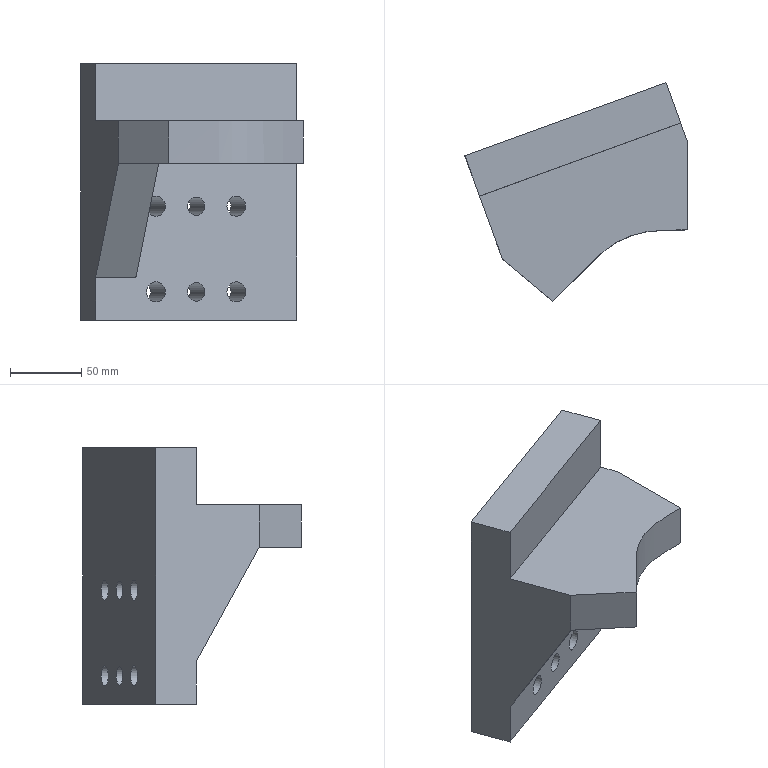Part | NX | features solid 2 | 1 solid | 20 faces | box 155.712 x 153.116 x 180 mm | volume 1134796 mm3 | plane 13 | cylinder 6 | spline 1 | commonest cylinder face diameters 14 x4 13 x2
STEP:
#1=CARTESIAN_POINT('',(-306.343,587.042,-175.));
#2=VERTEX_POINT('',#1);
#3=CARTESIAN_POINT('',(-300.235,589.265,-175.));
#4=DIRECTION('',(-0.342,0.9397,0.));
#5=DIRECTION('',(-0.9397,-0.342,0.));
#6=AXIS2_PLACEMENT_3D('',#3,#4,#5);
#7=CIRCLE('',#6,6.5);
#8=EDGE_CURVE('',#2,#2,#7,.F.);
#9=ORIENTED_EDGE('',*,*,#8,.T.);
#10=EDGE_LOOP('',(#9));
#11=FACE_BOUND('',#10,.T.);
#12=CARTESIAN_POINT('',(-278.622,597.132,-115.));
#13=VERTEX_POINT('',#12);
#14=CARTESIAN_POINT('',(-272.044,599.526,-115.));
#15=DIRECTION('',(-0.342,0.9397,0.));
#16=DIRECTION('',(-0.9397,-0.342,0.));
#17=AXIS2_PLACEMENT_3D('',#14,#15,#16);
#18=CIRCLE('',#17,7.);
#19=EDGE_CURVE('',#13,#13,#18,.F.);
#20=ORIENTED_EDGE('',*,*,#19,.T.);
#21=EDGE_LOOP('',(#20));
#22=FACE_BOUND('',#21,.T.);
#23=CARTESIAN_POINT('',(-335.003,576.611,-115.));
#24=VERTEX_POINT('',#23);
#25=CARTESIAN_POINT('',(-328.425,579.005,-115.));
#26=DIRECTION('',(-0.342,0.9397,0.));
#27=DIRECTION('',(-0.9397,-0.342,0.));
#28=AXIS2_PLACEMENT_3D('',#25,#26,#27);
#29=CIRCLE('',#28,7.);
#30=EDGE_CURVE('',#24,#24,#29,.F.);
#31=ORIENTED_EDGE('',*,*,#30,.T.);
#32=EDGE_LOOP('',(#31));
#33=FACE_BOUND('',#32,.T.);
#34=CARTESIAN_POINT('',(-370.712,563.614,-195.));
#35=VERTEX_POINT('',#34);
#36=CARTESIAN_POINT('',(-229.758,614.917,-195.));
#37=VERTEX_POINT('',#36);
#38=CARTESIAN_POINT('',(-389.448,556.794,-195.));
#39=DIRECTION('',(-0.9397,-0.342,0.));
#40=VECTOR('',#39,1000.);
#41=LINE('',#38,#40);
#42=EDGE_CURVE('',#35,#37,#41,.F.);
#43=ORIENTED_EDGE('',*,*,#42,.F.);
#44=CARTESIAN_POINT('',(-370.712,563.614,-15.));
#45=VERTEX_POINT('',#44);
#46=CARTESIAN_POINT('',(-370.712,563.614,-25.));
#47=DIRECTION('',(0.,0.,1.));
#48=VECTOR('',#47,1000.);
#49=LINE('',#46,#48);
#50=EDGE_CURVE('',#45,#35,#49,.F.);
#51=ORIENTED_EDGE('',*,*,#50,.F.);
#52=CARTESIAN_POINT('',(-229.758,614.917,-15.));
#53=VERTEX_POINT('',#52);
#54=CARTESIAN_POINT('',(-389.448,556.794,-15.));
#55=DIRECTION('',(0.9397,0.342,0.));
#56=VECTOR('',#55,1000.);
#57=LINE('',#54,#56);
#58=EDGE_CURVE('',#45,#53,#57,.T.);
#59=ORIENTED_EDGE('',*,*,#58,.T.);
#60=CARTESIAN_POINT('',(-229.758,614.917,-25.));
#61=DIRECTION('',(0.,0.,-1.));
#62=VECTOR('',#61,1000.);
#63=LINE('',#60,#62);
#64=EDGE_CURVE('',#53,#37,#63,.T.);
#65=ORIENTED_EDGE('',*,*,#64,.T.);
#66=EDGE_LOOP('',(#43,#51,#59,#65));
#67=FACE_BOUND('',#66,.T.);
#68=CARTESIAN_POINT('',(-306.343,587.042,-115.));
#69=VERTEX_POINT('',#68);
#70=CARTESIAN_POINT('',(-300.235,589.265,-115.));
#71=DIRECTION('',(-0.342,0.9397,0.));
#72=DIRECTION('',(-0.9397,-0.342,0.));
#73=AXIS2_PLACEMENT_3D('',#70,#71,#72);
#74=CIRCLE('',#73,6.5);
#75=EDGE_CURVE('',#69,#69,#74,.F.);
#76=ORIENTED_EDGE('',*,*,#75,.T.);
#77=EDGE_LOOP('',(#76));
#78=FACE_BOUND('',#77,.T.);
#79=CARTESIAN_POINT('',(-335.003,576.611,-175.));
#80=VERTEX_POINT('',#79);
#81=CARTESIAN_POINT('',(-328.425,579.005,-175.));
#82=DIRECTION('',(-0.342,0.9397,0.));
#83=DIRECTION('',(-0.9397,-0.342,0.));
#84=AXIS2_PLACEMENT_3D('',#81,#82,#83);
#85=CIRCLE('',#84,7.);
#86=EDGE_CURVE('',#80,#80,#85,.F.);
#87=ORIENTED_EDGE('',*,*,#86,.T.);
#88=EDGE_LOOP('',(#87));
#89=FACE_BOUND('',#88,.T.);
#90=CARTESIAN_POINT('',(-278.622,597.132,-175.));
#91=VERTEX_POINT('',#90);
#92=CARTESIAN_POINT('',(-272.044,599.526,-175.));
#93=DIRECTION('',(-0.342,0.9397,0.));
#94=DIRECTION('',(-0.9397,-0.342,0.));
#95=AXIS2_PLACEMENT_3D('',#92,#93,#94);
#96=CIRCLE('',#95,7.);
#97=EDGE_CURVE('',#91,#91,#96,.F.);
#98=ORIENTED_EDGE('',*,*,#97,.T.);
#99=EDGE_LOOP('',(#98));
#100=FACE_BOUND('',#99,.T.);
#101=CARTESIAN_POINT('',(-389.448,556.794,-25.));
#102=DIRECTION('',(-0.342,0.9397,0.));
#103=DIRECTION('',(-0.9397,-0.342,0.));
#104=AXIS2_PLACEMENT_3D('',#101,#102,#103);
#105=PLANE('',#104);
#106=ADVANCED_FACE('',(#11,#22,#33,#67,#78,#89,#100),#105,.T.);
#107=CARTESIAN_POINT('',(-296.082,558.852,-175.));
#108=VERTEX_POINT('',#107);
#109=CARTESIAN_POINT('',(-289.974,561.075,-175.));
#110=DIRECTION('',(-0.342,0.9397,0.));
#111=DIRECTION('',(-0.9397,-0.342,0.));
#112=AXIS2_PLACEMENT_3D('',#109,#110,#111);
#113=CIRCLE('',#112,6.5);
#114=EDGE_CURVE('',#108,#108,#113,.F.);
#115=ORIENTED_EDGE('',*,*,#114,.F.);
#116=EDGE_LOOP('',(#115));
#117=FACE_BOUND('',#116,.T.);
#118=CARTESIAN_POINT('',(-268.361,568.941,-115.));
#119=VERTEX_POINT('',#118);
#120=CARTESIAN_POINT('',(-261.783,571.335,-115.));
#121=DIRECTION('',(-0.342,0.9397,0.));
#122=DIRECTION('',(-0.9397,-0.342,0.));
#123=AXIS2_PLACEMENT_3D('',#120,#121,#122);
#124=CIRCLE('',#123,7.);
#125=EDGE_CURVE('',#119,#119,#124,.F.);
#126=ORIENTED_EDGE('',*,*,#125,.F.);
#127=EDGE_LOOP('',(#126));
#128=FACE_BOUND('',#127,.T.);
#129=CARTESIAN_POINT('',(-324.743,548.42,-115.));
#130=VERTEX_POINT('',#129);
#131=CARTESIAN_POINT('',(-318.165,550.814,-115.));
#132=DIRECTION('',(-0.342,0.9397,0.));
#133=DIRECTION('',(-0.9397,-0.342,0.));
#134=AXIS2_PLACEMENT_3D('',#131,#132,#133);
#135=CIRCLE('',#134,7.);
#136=EDGE_CURVE('',#130,#130,#135,.F.);
#137=ORIENTED_EDGE('',*,*,#136,.F.);
#138=EDGE_LOOP('',(#137));
#139=FACE_BOUND('',#138,.T.);
#140=CARTESIAN_POINT('',(-332.26,545.684,-85.));
#141=VERTEX_POINT('',#140);
#142=CARTESIAN_POINT('',(-219.497,586.726,-85.));
#143=VERTEX_POINT('',#142);
#144=CARTESIAN_POINT('',(-379.188,528.604,-85.));
#145=DIRECTION('',(0.9397,0.342,0.));
#146=VECTOR('',#145,1000.);
#147=LINE('',#144,#146);
#148=EDGE_CURVE('',#141,#143,#147,.T.);
#149=ORIENTED_EDGE('',*,*,#148,.F.);
#150=CARTESIAN_POINT('',(-332.26,545.684,-165.));
#151=VERTEX_POINT('',#150);
#152=CARTESIAN_POINT('',(-332.26,545.684,-85.));
#153=DIRECTION('',(0.,0.,1.));
#154=VECTOR('',#153,1000.);
#155=LINE('',#152,#154);
#156=EDGE_CURVE('',#141,#151,#155,.F.);
#157=ORIENTED_EDGE('',*,*,#156,.T.);
#158=CARTESIAN_POINT('',(-360.451,535.423,-165.));
#159=VERTEX_POINT('',#158);
#160=CARTESIAN_POINT('',(-360.451,535.423,-165.));
#161=DIRECTION('',(0.9397,0.342,0.));
#162=VECTOR('',#161,1000.);
#163=LINE('',#160,#162);
#164=EDGE_CURVE('',#159,#151,#163,.T.);
#165=ORIENTED_EDGE('',*,*,#164,.F.);
#166=CARTESIAN_POINT('',(-360.451,535.423,-195.));
#167=VERTEX_POINT('',#166);
#168=CARTESIAN_POINT('',(-360.451,535.423,-25.));
#169=DIRECTION('',(0.,0.,1.));
#170=VECTOR('',#169,1000.);
#171=LINE('',#168,#170);
#172=EDGE_CURVE('',#159,#167,#171,.F.);
#173=ORIENTED_EDGE('',*,*,#172,.T.);
#174=CARTESIAN_POINT('',(-219.497,586.726,-195.));
#175=VERTEX_POINT('',#174);
#176=CARTESIAN_POINT('',(-379.188,528.604,-195.));
#177=DIRECTION('',(-0.9397,-0.342,0.));
#178=VECTOR('',#177,1000.);
#179=LINE('',#176,#178);
#180=EDGE_CURVE('',#167,#175,#179,.F.);
#181=ORIENTED_EDGE('',*,*,#180,.T.);
#182=CARTESIAN_POINT('',(-219.497,586.726,-25.));
#183=DIRECTION('',(0.,0.,-1.));
#184=VECTOR('',#183,1000.);
#185=LINE('',#182,#184);
#186=EDGE_CURVE('',#143,#175,#185,.T.);
#187=ORIENTED_EDGE('',*,*,#186,.F.);
#188=EDGE_LOOP('',(#149,#157,#165,#173,#181,#187));
#189=FACE_BOUND('',#188,.T.);
#190=CARTESIAN_POINT('',(-296.082,558.852,-115.));
#191=VERTEX_POINT('',#190);
#192=CARTESIAN_POINT('',(-289.974,561.075,-115.));
#193=DIRECTION('',(-0.342,0.9397,0.));
#194=DIRECTION('',(-0.9397,-0.342,0.));
#195=AXIS2_PLACEMENT_3D('',#192,#193,#194);
#196=CIRCLE('',#195,6.5);
#197=EDGE_CURVE('',#191,#191,#196,.F.);
#198=ORIENTED_EDGE('',*,*,#197,.F.);
#199=EDGE_LOOP('',(#198));
#200=FACE_BOUND('',#199,.T.);
#201=CARTESIAN_POINT('',(-324.743,548.42,-175.));
#202=VERTEX_POINT('',#201);
#203=CARTESIAN_POINT('',(-318.165,550.814,-175.));
#204=DIRECTION('',(-0.342,0.9397,0.));
#205=DIRECTION('',(-0.9397,-0.342,0.));
#206=AXIS2_PLACEMENT_3D('',#203,#204,#205);
#207=CIRCLE('',#206,7.);
#208=EDGE_CURVE('',#202,#202,#207,.F.);
#209=ORIENTED_EDGE('',*,*,#208,.F.);
#210=EDGE_LOOP('',(#209));
#211=FACE_BOUND('',#210,.T.);
#212=CARTESIAN_POINT('',(-268.361,568.941,-175.));
#213=VERTEX_POINT('',#212);
#214=CARTESIAN_POINT('',(-261.783,571.335,-175.));
#215=DIRECTION('',(-0.342,0.9397,0.));
#216=DIRECTION('',(-0.9397,-0.342,0.));
#217=AXIS2_PLACEMENT_3D('',#214,#215,#216);
#218=CIRCLE('',#217,7.);
#219=EDGE_CURVE('',#213,#213,#218,.F.);
#220=ORIENTED_EDGE('',*,*,#219,.F.);
#221=EDGE_LOOP('',(#220));
#222=FACE_BOUND('',#221,.T.);
#223=CARTESIAN_POINT('',(-379.188,528.604,-25.));
#224=DIRECTION('',(-0.342,0.9397,0.));
#225=DIRECTION('',(-0.9397,-0.342,0.));
#226=AXIS2_PLACEMENT_3D('',#223,#224,#225);
#227=PLANE('',#226);
#228=ADVANCED_FACE('',(#117,#128,#139,#189,#200,#211,#222),#227,.F.);
#229=CARTESIAN_POINT('',(-360.451,535.423,-55.));
#230=VERTEX_POINT('',#229);
#231=CARTESIAN_POINT('',(-219.497,586.726,-55.));
#232=VERTEX_POINT('',#231);
#233=CARTESIAN_POINT('',(-379.188,528.604,-55.));
#234=DIRECTION('',(0.9397,0.342,0.));
#235=VECTOR('',#234,1000.);
#236=LINE('',#233,#235);
#237=EDGE_CURVE('',#230,#232,#236,.T.);
#238=ORIENTED_EDGE('',*,*,#237,.T.);
#239=CARTESIAN_POINT('',(-219.497,586.726,-15.));
#240=VERTEX_POINT('',#239);
#241=CARTESIAN_POINT('',(-219.497,586.726,-25.));
#242=DIRECTION('',(0.,0.,-1.));
#243=VECTOR('',#242,1000.);
#244=LINE('',#241,#243);
#245=EDGE_CURVE('',#240,#232,#244,.T.);
#246=ORIENTED_EDGE('',*,*,#245,.F.);
#247=CARTESIAN_POINT('',(-360.451,535.423,-15.));
#248=VERTEX_POINT('',#247);
#249=CARTESIAN_POINT('',(-379.188,528.604,-15.));
#250=DIRECTION('',(0.9397,0.342,0.));
#251=VECTOR('',#250,1000.);
#252=LINE('',#249,#251);
#253=EDGE_CURVE('',#248,#240,#252,.T.);
#254=ORIENTED_EDGE('',*,*,#253,.F.);
#255=CARTESIAN_POINT('',(-360.451,535.423,-25.));
#256=DIRECTION('',(0.,0.,1.));
#257=VECTOR('',#256,1000.);
#258=LINE('',#255,#257);
#259=EDGE_CURVE('',#248,#230,#258,.F.);
#260=ORIENTED_EDGE('',*,*,#259,.T.);
#261=EDGE_LOOP('',(#238,#246,#254,#260));
#262=FACE_BOUND('',#261,.T.);
#263=CARTESIAN_POINT('',(-379.188,528.604,-25.));
#264=DIRECTION('',(-0.342,0.9397,0.));
#265=DIRECTION('',(-0.9397,-0.342,0.));
#266=AXIS2_PLACEMENT_3D('',#263,#264,#265);
#267=PLANE('',#266);
#268=ADVANCED_FACE('',(#262),#267,.F.);
#269=CARTESIAN_POINT('',(-367.291,554.217,-15.));
#270=DIRECTION('',(0.342,-0.9397,0.));
#271=VECTOR('',#270,1000.);
#272=LINE('',#269,#271);
#273=EDGE_CURVE('',#248,#45,#272,.F.);
#274=ORIENTED_EDGE('',*,*,#273,.F.);
#275=ORIENTED_EDGE('',*,*,#253,.T.);
#276=CARTESIAN_POINT('',(-226.338,605.52,-15.));
#277=DIRECTION('',(-0.342,0.9397,0.));
#278=VECTOR('',#277,1000.);
#279=LINE('',#276,#278);
#280=EDGE_CURVE('',#240,#53,#279,.T.);
#281=ORIENTED_EDGE('',*,*,#280,.T.);
#282=ORIENTED_EDGE('',*,*,#58,.F.);
#283=EDGE_LOOP('',(#274,#275,#281,#282));
#284=FACE_BOUND('',#283,.T.);
#285=CARTESIAN_POINT('',(-386.028,547.397,-15.));
#286=DIRECTION('',(0.,0.,1.));
#287=DIRECTION('',(0.9397,0.342,0.));
#288=AXIS2_PLACEMENT_3D('',#285,#286,#287);
#289=PLANE('',#288);
#290=ADVANCED_FACE('',(#284),#289,.T.);
#291=CARTESIAN_POINT('',(-215.,574.37,-85.));
#292=VERTEX_POINT('',#291);
#293=CARTESIAN_POINT('',(-215.,574.37,-55.));
#294=VERTEX_POINT('',#293);
#295=CARTESIAN_POINT('',(-215.,574.37,-25.));
#296=DIRECTION('',(0.,0.,1.));
#297=VECTOR('',#296,1000.);
#298=LINE('',#295,#297);
#299=EDGE_CURVE('',#292,#294,#298,.T.);
#300=ORIENTED_EDGE('',*,*,#299,.F.);
#301=CARTESIAN_POINT('',(-226.338,605.52,-85.));
#302=DIRECTION('',(0.342,-0.9397,0.));
#303=VECTOR('',#302,1000.);
#304=LINE('',#301,#303);
#305=EDGE_CURVE('',#143,#292,#304,.T.);
#306=ORIENTED_EDGE('',*,*,#305,.F.);
#307=ORIENTED_EDGE('',*,*,#186,.T.);
#308=CARTESIAN_POINT('',(-136.812,359.551,-195.));
#309=DIRECTION('',(0.342,-0.9397,0.));
#310=VECTOR('',#309,1000.);
#311=LINE('',#308,#310);
#312=EDGE_CURVE('',#175,#37,#311,.F.);
#313=ORIENTED_EDGE('',*,*,#312,.T.);
#314=ORIENTED_EDGE('',*,*,#64,.F.);
#315=ORIENTED_EDGE('',*,*,#280,.F.);
#316=ORIENTED_EDGE('',*,*,#245,.T.);
#317=CARTESIAN_POINT('',(-226.338,605.52,-55.));
#318=DIRECTION('',(0.342,-0.9397,0.));
#319=VECTOR('',#318,1000.);
#320=LINE('',#317,#319);
#321=EDGE_CURVE('',#232,#294,#320,.T.);
#322=ORIENTED_EDGE('',*,*,#321,.T.);
#323=EDGE_LOOP('',(#300,#306,#307,#313,#314,#315,#316,#322));
#324=FACE_BOUND('',#323,.T.);
#325=CARTESIAN_POINT('',(-136.812,359.551,-25.));
#326=DIRECTION('',(0.9397,0.342,0.));
#327=DIRECTION('',(-0.342,0.9397,0.));
#328=AXIS2_PLACEMENT_3D('',#325,#326,#327);
#329=PLANE('',#328);
#330=ADVANCED_FACE('',(#324),#329,.T.);
#331=ORIENTED_EDGE('',*,*,#312,.F.);
#332=ORIENTED_EDGE('',*,*,#180,.F.);
#333=CARTESIAN_POINT('',(-367.291,554.217,-195.));
#334=DIRECTION('',(-0.342,0.9397,0.));
#335=VECTOR('',#334,1000.);
#336=LINE('',#333,#335);
#337=EDGE_CURVE('',#167,#35,#336,.T.);
#338=ORIENTED_EDGE('',*,*,#337,.T.);
#339=ORIENTED_EDGE('',*,*,#42,.T.);
#340=EDGE_LOOP('',(#331,#332,#338,#339));
#341=FACE_BOUND('',#340,.T.);
#342=CARTESIAN_POINT('',(-386.028,547.397,-195.));
#343=DIRECTION('',(0.,0.,1.));
#344=DIRECTION('',(0.9397,0.342,0.));
#345=AXIS2_PLACEMENT_3D('',#342,#343,#344);
#346=PLANE('',#345);
#347=ADVANCED_FACE('',(#341),#346,.F.);
#348=ORIENTED_EDGE('',*,*,#172,.F.);
#349=CARTESIAN_POINT('',(-344.4,491.324,-85.));
#350=VERTEX_POINT('',#349);
#351=CARTESIAN_POINT('',(-348.51,502.614,-105.481));
#352=DIRECTION('',(-0.1731,0.4755,-0.8625));
#353=VECTOR('',#352,1000.);
#354=LINE('',#351,#353);
#355=EDGE_CURVE('',#350,#159,#354,.T.);
#356=ORIENTED_EDGE('',*,*,#355,.F.);
#357=CARTESIAN_POINT('',(-344.4,491.324,-55.));
#358=VERTEX_POINT('',#357);
#359=CARTESIAN_POINT('',(-344.4,491.324,-25.));
#360=DIRECTION('',(0.,0.,1.));
#361=VECTOR('',#360,1000.);
#362=LINE('',#359,#361);
#363=EDGE_CURVE('',#358,#350,#362,.F.);
#364=ORIENTED_EDGE('',*,*,#363,.F.);
#365=CARTESIAN_POINT('',(-367.291,554.217,-55.));
#366=DIRECTION('',(-0.342,0.9397,0.));
#367=VECTOR('',#366,1000.);
#368=LINE('',#365,#367);
#369=EDGE_CURVE('',#230,#358,#368,.F.);
#370=ORIENTED_EDGE('',*,*,#369,.F.);
#371=ORIENTED_EDGE('',*,*,#259,.F.);
#372=ORIENTED_EDGE('',*,*,#273,.T.);
#373=ORIENTED_EDGE('',*,*,#50,.T.);
#374=ORIENTED_EDGE('',*,*,#337,.F.);
#375=EDGE_LOOP('',(#348,#356,#364,#370,#371,#372,#373,#374));
#376=FACE_BOUND('',#375,.T.);
#377=CARTESIAN_POINT('',(-367.291,554.217,-25.));
#378=DIRECTION('',(0.9397,0.342,0.));
#379=DIRECTION('',(-0.342,0.9397,0.));
#380=AXIS2_PLACEMENT_3D('',#377,#378,#379);
#381=PLANE('',#380);
#382=ADVANCED_FACE('',(#376),#381,.F.);
#383=CARTESIAN_POINT('',(-309.215,461.801,-85.));
#384=VERTEX_POINT('',#383);
#385=CARTESIAN_POINT('',(-215.,511.787,-85.));
#386=VERTEX_POINT('',#385);
#387=CARTESIAN_POINT('',(-309.215,461.801,-85.));
#388=CARTESIAN_POINT('',(-305.882,465.082,-85.));
#389=CARTESIAN_POINT('',(-299.215,471.644,-85.));
#390=CARTESIAN_POINT('',(-290.855,479.819,-85.));
#391=CARTESIAN_POINT('',(-284.22,486.416,-85.));
#392=CARTESIAN_POINT('',(-279.319,491.432,-85.));
#393=CARTESIAN_POINT('',(-274.205,496.261,-85.));
#394=CARTESIAN_POINT('',(-268.737,500.555,-85.));
#395=CARTESIAN_POINT('',(-262.837,504.142,-85.));
#396=CARTESIAN_POINT('',(-254.308,508.012,-85.));
#397=CARTESIAN_POINT('',(-243.046,511.013,-85.));
#398=CARTESIAN_POINT('',(-229.004,511.804,-85.));
#399=CARTESIAN_POINT('',(-219.67,511.778,-85.));
#400=CARTESIAN_POINT('',(-215.,511.787,-85.));
#401=B_SPLINE_CURVE_WITH_KNOTS('',3,(#387,#388,#389,#390,#391,#392,#393,#394,#395,#396,#397,#398,#399,#400),.UNSPECIFIED.,.F.,.F.,(4,1,1,1,1,1,1,1,1,1,1,4),(0.6899,0.704,0.718,0.725,0.732,0.7391,0.7461,0.7531,0.7601,0.7741,0.7882,0.8022),.UNSPECIFIED.);
#402=EDGE_CURVE('',#384,#386,#401,.T.);
#403=ORIENTED_EDGE('',*,*,#402,.T.);
#404=CARTESIAN_POINT('',(-215.,511.787,-55.));
#405=VERTEX_POINT('',#404);
#406=CARTESIAN_POINT('',(-215.,511.787,-85.));
#407=CARTESIAN_POINT('',(-215.,511.787,-75.));
#408=CARTESIAN_POINT('',(-215.,511.787,-65.));
#409=CARTESIAN_POINT('',(-215.,511.787,-55.));
#410=B_SPLINE_CURVE_WITH_KNOTS('',3,(#406,#407,#408,#409),.UNSPECIFIED.,.F.,.F.,(4,4),(0.,0.03),.UNSPECIFIED.);
#411=EDGE_CURVE('',#386,#405,#410,.T.);
#412=ORIENTED_EDGE('',*,*,#411,.T.);
#413=CARTESIAN_POINT('',(-309.215,461.801,-55.));
#414=VERTEX_POINT('',#413);
#415=CARTESIAN_POINT('',(-309.215,461.801,-55.));
#416=CARTESIAN_POINT('',(-305.922,465.042,-55.));
#417=CARTESIAN_POINT('',(-299.335,471.525,-55.));
#418=CARTESIAN_POINT('',(-291.079,479.603,-55.));
#419=CARTESIAN_POINT('',(-284.515,486.115,-55.));
#420=CARTESIAN_POINT('',(-278.051,492.743,-55.));
#421=CARTESIAN_POINT('',(-271.233,498.96,-55.));
#422=CARTESIAN_POINT('',(-263.34,503.881,-55.));
#423=CARTESIAN_POINT('',(-254.631,507.911,-55.));
#424=CARTESIAN_POINT('',(-243.376,510.964,-55.));
#425=CARTESIAN_POINT('',(-229.212,511.809,-55.));
#426=CARTESIAN_POINT('',(-219.735,511.778,-55.));
#427=CARTESIAN_POINT('',(-215.,511.787,-55.));
#428=B_SPLINE_CURVE_WITH_KNOTS('',3,(#415,#416,#417,#418,#419,#420,#421,#422,#423,#424,#425,#426,#427),.UNSPECIFIED.,.F.,.F.,(4,1,1,1,1,1,1,1,1,1,4),(0.02527,0.03913,0.05299,0.05992,0.06686,0.08072,0.08765,0.09458,0.1084,0.1223,0.1362),.UNSPECIFIED.);
#429=EDGE_CURVE('',#414,#405,#428,.T.);
#430=ORIENTED_EDGE('',*,*,#429,.F.);
#431=CARTESIAN_POINT('',(-309.215,461.801,-55.));
#432=CARTESIAN_POINT('',(-309.215,461.801,-65.));
#433=CARTESIAN_POINT('',(-309.215,461.801,-75.));
#434=CARTESIAN_POINT('',(-309.215,461.801,-85.));
#435=B_SPLINE_CURVE_WITH_KNOTS('',3,(#431,#432,#433,#434),.UNSPECIFIED.,.F.,.F.,(4,4),(0.,0.03),.UNSPECIFIED.);
#436=EDGE_CURVE('',#414,#384,#435,.T.);
#437=ORIENTED_EDGE('',*,*,#436,.T.);
#438=EDGE_LOOP('',(#403,#412,#430,#437));
#439=FACE_BOUND('',#438,.T.);
#440=CARTESIAN_POINT('',(-309.215,461.801,-55.));
#441=CARTESIAN_POINT('',(-309.215,461.801,-85.));
#442=CARTESIAN_POINT('',(-306.004,464.961,-55.));
#443=CARTESIAN_POINT('',(-306.004,464.961,-85.));
#444=CARTESIAN_POINT('',(-299.588,471.274,-55.));
#445=CARTESIAN_POINT('',(-299.588,471.274,-85.));
#446=CARTESIAN_POINT('',(-291.532,479.162,-55.));
#447=CARTESIAN_POINT('',(-291.532,479.162,-85.));
#448=CARTESIAN_POINT('',(-285.185,485.443,-55.));
#449=CARTESIAN_POINT('',(-285.185,485.443,-85.));
#450=CARTESIAN_POINT('',(-280.483,490.251,-55.));
#451=CARTESIAN_POINT('',(-280.483,490.251,-85.));
#452=CARTESIAN_POINT('',(-275.447,495.157,-55.));
#453=CARTESIAN_POINT('',(-275.447,495.157,-85.));
#454=CARTESIAN_POINT('',(-269.825,499.801,-55.));
#455=CARTESIAN_POINT('',(-269.825,499.801,-85.));
#456=CARTESIAN_POINT('',(-263.533,503.793,-55.));
#457=CARTESIAN_POINT('',(-263.533,503.793,-85.));
#458=CARTESIAN_POINT('',(-256.85,506.896,-55.));
#459=CARTESIAN_POINT('',(-256.85,506.896,-85.));
#460=CARTESIAN_POINT('',(-249.894,509.202,-55.));
#461=CARTESIAN_POINT('',(-249.894,509.202,-85.));
#462=CARTESIAN_POINT('',(-240.326,511.212,-55.));
#463=CARTESIAN_POINT('',(-240.326,511.212,-85.));
#464=CARTESIAN_POINT('',(-228.488,511.796,-55.));
#465=CARTESIAN_POINT('',(-228.488,511.796,-85.));
#466=CARTESIAN_POINT('',(-219.522,511.779,-55.));
#467=CARTESIAN_POINT('',(-219.522,511.779,-85.));
#468=CARTESIAN_POINT('',(-215.,511.787,-55.));
#469=CARTESIAN_POINT('',(-215.,511.787,-85.));
#470=B_SPLINE_SURFACE_WITH_KNOTS('',3,1,((#440,#441),(#442,#443),(#444,#445),(#446,#447),(#448,#449),(#450,#451),(#452,#453),(#454,#455),(#456,#457),(#458,#459),(#460,#461),(#462,#463),(#464,#465),(#466,#467),(#468,#469)),.SURF_OF_LINEAR_EXTRUSION.,.F.,.F.,.F.,(4,1,1,1,1,1,1,1,1,1,1,1,4),(2,2),(0.06481,0.1563,0.2478,0.2936,0.3393,0.3851,0.4308,0.4766,0.5223,0.5681,0.6138,0.7053,0.7968),(0.,1.),.UNSPECIFIED.);
#471=ADVANCED_FACE('',(#439),#470,.F.);
#472=CARTESIAN_POINT('',(-316.21,501.585,-85.));
#473=VERTEX_POINT('',#472);
#474=CARTESIAN_POINT('',(-332.26,545.684,-85.));
#475=DIRECTION('',(-0.342,0.9397,0.));
#476=VECTOR('',#475,1000.);
#477=LINE('',#474,#476);
#478=EDGE_CURVE('',#141,#473,#477,.F.);
#479=ORIENTED_EDGE('',*,*,#478,.F.);
#480=ORIENTED_EDGE('',*,*,#148,.T.);
#481=ORIENTED_EDGE('',*,*,#305,.T.);
#482=CARTESIAN_POINT('',(-215.,547.397,-85.));
#483=DIRECTION('',(0.,1.,0.));
#484=VECTOR('',#483,1000.);
#485=LINE('',#482,#484);
#486=EDGE_CURVE('',#386,#292,#485,.T.);
#487=ORIENTED_EDGE('',*,*,#486,.F.);
#488=ORIENTED_EDGE('',*,*,#402,.F.);
#489=CARTESIAN_POINT('',(-396.439,534.99,-85.));
#490=DIRECTION('',(0.766,-0.6428,0.));
#491=VECTOR('',#490,1000.);
#492=LINE('',#489,#491);
#493=EDGE_CURVE('',#350,#384,#492,.T.);
#494=ORIENTED_EDGE('',*,*,#493,.F.);
#495=CARTESIAN_POINT('',(-344.4,491.324,-85.));
#496=DIRECTION('',(-0.9397,-0.342,0.));
#497=VECTOR('',#496,1000.);
#498=LINE('',#495,#497);
#499=EDGE_CURVE('',#350,#473,#498,.F.);
#500=ORIENTED_EDGE('',*,*,#499,.T.);
#501=EDGE_LOOP('',(#479,#480,#481,#487,#488,#494,#500));
#502=FACE_BOUND('',#501,.T.);
#503=CARTESIAN_POINT('',(-386.028,547.397,-85.));
#504=DIRECTION('',(0.,0.,-1.));
#505=DIRECTION('',(-0.6554,0.7553,0.));
#506=AXIS2_PLACEMENT_3D('',#503,#504,#505);
#507=PLANE('',#506);
#508=ADVANCED_FACE('',(#502),#507,.T.);
#509=ORIENTED_EDGE('',*,*,#429,.T.);
#510=CARTESIAN_POINT('',(-215.,547.397,-55.));
#511=DIRECTION('',(0.,1.,0.));
#512=VECTOR('',#511,1000.);
#513=LINE('',#510,#512);
#514=EDGE_CURVE('',#405,#294,#513,.T.);
#515=ORIENTED_EDGE('',*,*,#514,.T.);
#516=ORIENTED_EDGE('',*,*,#321,.F.);
#517=ORIENTED_EDGE('',*,*,#237,.F.);
#518=ORIENTED_EDGE('',*,*,#369,.T.);
#519=CARTESIAN_POINT('',(-396.439,534.99,-55.));
#520=DIRECTION('',(0.766,-0.6428,0.));
#521=VECTOR('',#520,1000.);
#522=LINE('',#519,#521);
#523=EDGE_CURVE('',#358,#414,#522,.T.);
#524=ORIENTED_EDGE('',*,*,#523,.T.);
#525=EDGE_LOOP('',(#509,#515,#516,#517,#518,#524));
#526=FACE_BOUND('',#525,.T.);
#527=CARTESIAN_POINT('',(-386.028,547.397,-55.));
#528=DIRECTION('',(0.,0.,-1.));
#529=DIRECTION('',(-0.6554,0.7553,0.));
#530=AXIS2_PLACEMENT_3D('',#527,#528,#529);
#531=PLANE('',#530);
#532=ADVANCED_FACE('',(#526),#531,.F.);
#533=ORIENTED_EDGE('',*,*,#30,.F.);
#534=EDGE_LOOP('',(#533));
#535=FACE_BOUND('',#534,.T.);
#536=ORIENTED_EDGE('',*,*,#136,.T.);
#537=EDGE_LOOP('',(#536));
#538=FACE_BOUND('',#537,.T.);
#539=CARTESIAN_POINT('',(-369.468,691.768,-115.));
#540=DIRECTION('',(0.342,-0.9397,0.));
#541=DIRECTION('',(0.9397,0.342,0.));
#542=AXIS2_PLACEMENT_3D('',#539,#540,#541);
#543=CYLINDRICAL_SURFACE('',#542,7.);
#544=ADVANCED_FACE('',(#535,#538),#543,.F.);
#545=ORIENTED_EDGE('',*,*,#75,.F.);
#546=EDGE_LOOP('',(#545));
#547=FACE_BOUND('',#546,.T.);
#548=ORIENTED_EDGE('',*,*,#197,.T.);
#549=EDGE_LOOP('',(#548));
#550=FACE_BOUND('',#549,.T.);
#551=CARTESIAN_POINT('',(-341.277,702.029,-115.));
#552=DIRECTION('',(0.342,-0.9397,0.));
#553=DIRECTION('',(0.9397,0.342,0.));
#554=AXIS2_PLACEMENT_3D('',#551,#552,#553);
#555=CYLINDRICAL_SURFACE('',#554,6.5);
#556=ADVANCED_FACE('',(#547,#550),#555,.F.);
#557=ORIENTED_EDGE('',*,*,#19,.F.);
#558=EDGE_LOOP('',(#557));
#559=FACE_BOUND('',#558,.T.);
#560=ORIENTED_EDGE('',*,*,#125,.T.);
#561=EDGE_LOOP('',(#560));
#562=FACE_BOUND('',#561,.T.);
#563=CARTESIAN_POINT('',(-313.086,712.289,-115.));
#564=DIRECTION('',(0.342,-0.9397,0.));
#565=DIRECTION('',(0.9397,0.342,0.));
#566=AXIS2_PLACEMENT_3D('',#563,#564,#565);
#567=CYLINDRICAL_SURFACE('',#566,7.);
#568=ADVANCED_FACE('',(#559,#562),#567,.F.);
#569=ORIENTED_EDGE('',*,*,#86,.F.);
#570=EDGE_LOOP('',(#569));
#571=FACE_BOUND('',#570,.T.);
#572=ORIENTED_EDGE('',*,*,#208,.T.);
#573=EDGE_LOOP('',(#572));
#574=FACE_BOUND('',#573,.T.);
#575=CARTESIAN_POINT('',(-369.468,691.768,-175.));
#576=DIRECTION('',(0.342,-0.9397,0.));
#577=DIRECTION('',(0.9397,0.342,0.));
#578=AXIS2_PLACEMENT_3D('',#575,#576,#577);
#579=CYLINDRICAL_SURFACE('',#578,7.);
#580=ADVANCED_FACE('',(#571,#574),#579,.F.);
#581=ORIENTED_EDGE('',*,*,#8,.F.);
#582=EDGE_LOOP('',(#581));
#583=FACE_BOUND('',#582,.T.);
#584=ORIENTED_EDGE('',*,*,#114,.T.);
#585=EDGE_LOOP('',(#584));
#586=FACE_BOUND('',#585,.T.);
#587=CARTESIAN_POINT('',(-341.277,702.029,-175.));
#588=DIRECTION('',(0.342,-0.9397,0.));
#589=DIRECTION('',(0.9397,0.342,0.));
#590=AXIS2_PLACEMENT_3D('',#587,#588,#589);
#591=CYLINDRICAL_SURFACE('',#590,6.5);
#592=ADVANCED_FACE('',(#583,#586),#591,.F.);
#593=ORIENTED_EDGE('',*,*,#97,.F.);
#594=EDGE_LOOP('',(#593));
#595=FACE_BOUND('',#594,.T.);
#596=ORIENTED_EDGE('',*,*,#219,.T.);
#597=EDGE_LOOP('',(#596));
#598=FACE_BOUND('',#597,.T.);
#599=CARTESIAN_POINT('',(-313.086,712.289,-175.));
#600=DIRECTION('',(0.342,-0.9397,0.));
#601=DIRECTION('',(0.9397,0.342,0.));
#602=AXIS2_PLACEMENT_3D('',#599,#600,#601);
#603=CYLINDRICAL_SURFACE('',#602,7.);
#604=ADVANCED_FACE('',(#595,#598),#603,.F.);
#605=ORIENTED_EDGE('',*,*,#493,.T.);
#606=ORIENTED_EDGE('',*,*,#436,.F.);
#607=ORIENTED_EDGE('',*,*,#523,.F.);
#608=ORIENTED_EDGE('',*,*,#363,.T.);
#609=EDGE_LOOP('',(#605,#606,#607,#608));
#610=FACE_BOUND('',#609,.T.);
#611=CARTESIAN_POINT('',(-359.995,504.409,-114.869));
#612=DIRECTION('',(0.6428,0.766,0.));
#613=DIRECTION('',(-0.766,0.6428,0.));
#614=AXIS2_PLACEMENT_3D('',#611,#612,#613);
#615=PLANE('',#614);
#616=ADVANCED_FACE('',(#610),#615,.F.);
#617=ORIENTED_EDGE('',*,*,#486,.T.);
#618=ORIENTED_EDGE('',*,*,#299,.T.);
#619=ORIENTED_EDGE('',*,*,#514,.F.);
#620=ORIENTED_EDGE('',*,*,#411,.F.);
#621=EDGE_LOOP('',(#617,#618,#619,#620));
#622=FACE_BOUND('',#621,.T.);
#623=CARTESIAN_POINT('',(-215.,550.,-157.5));
#624=DIRECTION('',(-1.,0.,0.));
#625=DIRECTION('',(0.,0.,1.));
#626=AXIS2_PLACEMENT_3D('',#623,#624,#625);
#627=PLANE('',#626);
#628=ADVANCED_FACE('',(#622),#627,.F.);
#629=ORIENTED_EDGE('',*,*,#478,.T.);
#630=CARTESIAN_POINT('',(-320.319,512.875,-105.481));
#631=DIRECTION('',(-0.1731,0.4755,-0.8625));
#632=VECTOR('',#631,1000.);
#633=LINE('',#630,#632);
#634=EDGE_CURVE('',#473,#151,#633,.T.);
#635=ORIENTED_EDGE('',*,*,#634,.T.);
#636=ORIENTED_EDGE('',*,*,#156,.F.);
#637=EDGE_LOOP('',(#629,#635,#636));
#638=FACE_BOUND('',#637,.T.);
#639=CARTESIAN_POINT('',(-332.26,545.684,-85.));
#640=DIRECTION('',(0.9397,0.342,0.));
#641=DIRECTION('',(-0.342,0.9397,0.));
#642=AXIS2_PLACEMENT_3D('',#639,#640,#641);
#643=PLANE('',#642);
#644=ADVANCED_FACE('',(#638),#643,.T.);
#645=ORIENTED_EDGE('',*,*,#634,.F.);
#646=ORIENTED_EDGE('',*,*,#499,.F.);
#647=ORIENTED_EDGE('',*,*,#355,.T.);
#648=ORIENTED_EDGE('',*,*,#164,.T.);
#649=EDGE_LOOP('',(#645,#646,#647,#648));
#650=FACE_BOUND('',#649,.T.);
#651=CARTESIAN_POINT('',(-360.451,535.423,-165.));
#652=DIRECTION('',(0.295,-0.8105,-0.506));
#653=DIRECTION('',(0.,0.5295,-0.8483));
#654=AXIS2_PLACEMENT_3D('',#651,#652,#653);
#655=PLANE('',#654);
#656=ADVANCED_FACE('',(#650),#655,.T.);
#657=CLOSED_SHELL('',(#106,#228,#268,#290,#330,#347,#382,#471,#508,#532,#544,#556,#568,#580,#592,#604,#616,#628,#644,#656));
#658=MANIFOLD_SOLID_BREP('',#657);
#659=(LENGTH_UNIT()NAMED_UNIT(*)SI_UNIT(.MILLI.,.METRE.));
#660=UNCERTAINTY_MEASURE_WITH_UNIT(LENGTH_MEASURE(0.0508),#659,'','');
#661=(NAMED_UNIT(*)PLANE_ANGLE_UNIT()SI_UNIT($,.RADIAN.));
#662=(NAMED_UNIT(*)SI_UNIT($,.STERADIAN.)SOLID_ANGLE_UNIT());
#663=(GEOMETRIC_REPRESENTATION_CONTEXT(3)GLOBAL_UNCERTAINTY_ASSIGNED_CONTEXT((#660))GLOBAL_UNIT_ASSIGNED_CONTEXT((#659,#661,#662))REPRESENTATION_CONTEXT('',''));
#664=ADVANCED_BREP_SHAPE_REPRESENTATION('',(#658),#663);